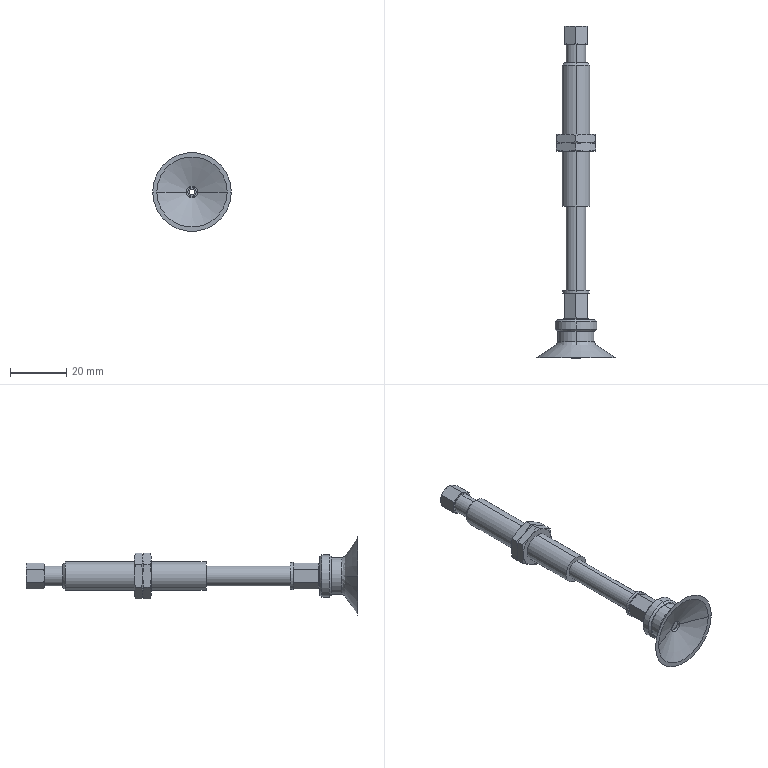Part | SolidWorks | features BaseBody 3 | 3 solids | 160 faces | box 28 x 118 x 28 mm | volume 8607 mm3 | cone 77 | plane 45 | cylinder 32 | spline 6 | commonest cylinder face diameters 5 x4 6 x4 7 x4 10 x4 2 x2 3 x2